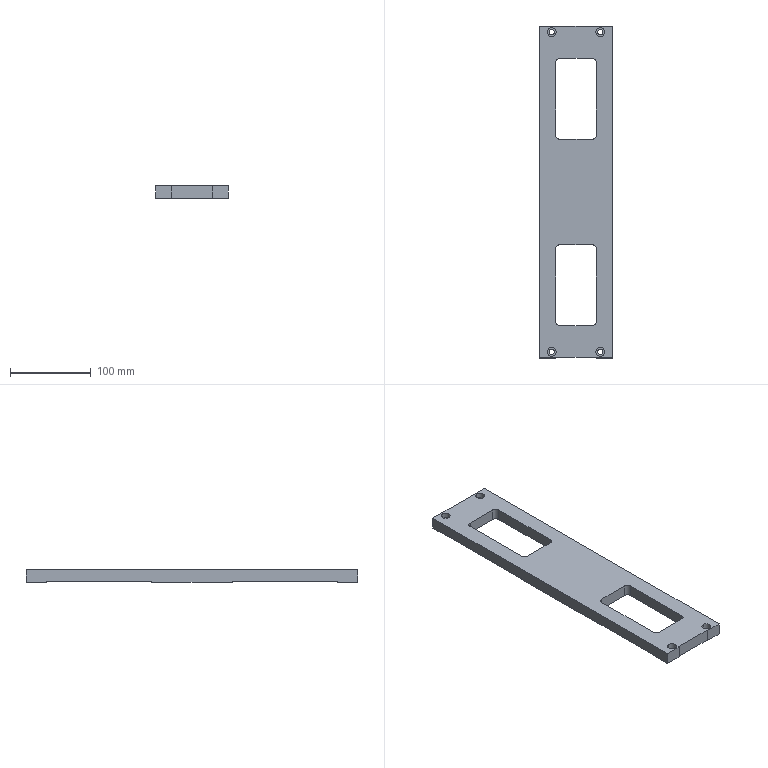NC program | NX | posted with a generic post | part box 90 x 410 x 15 mm
Lines 56 to 1434 of 4348:
(ZLEVEL_PROFILE , TOOL : D10)
N98 T10 M6
N100 G54
N102 G17 G0 G90 X209.1 Y-18.909 S9500 M3
N104 G43 Z30. H10
N106 Z1.5
N108 G94 G1 Y-21.967 Z1.34 F1000.
N110 X209.29 Y-22.224 Z1.323
N112 X209.699 Y-22.992 Z1.277
N114 X209.972 Y-23.819 Z1.232
N116 X210.1 Y-24.68 Z1.186
N118 Y-45.32 Z0.104
N120 X209.983 Y-46.131 Z0.062
N122 X209.738 Y-46.914 Z0.019
N124 X209.371 Y-47.647 Z-0.024
N126 X208.892 Y-48.312 Z-0.067
N128 X208.312 Y-48.892 Z-0.11
N130 X207.647 Y-49.371 Z-0.153
N132 X206.914 Y-49.738 Z-0.196
N134 X206.131 Y-49.983 Z-0.239
N136 X205.32 Y-50.1 Z-0.282
N138 X205. Z-0.299
N140 X-205. F3000.
N142 G2 X-210.1 Y-45. R5.1
N144 G1 Y45.
N146 G2 X-205. Y50.1 R5.1
N148 G1 X205.
N150 G2 X210.1 Y45. R5.1
N152 G1 Y25.
N154 G2 X209.1 Y21.967 R5.1
N156 G1 Y-21.967
N158 G2 X210.1 Y-25. R5.1
N160 G1 Y-45.
N162 G2 X205. Y-50.1 R5.1
N164 G1 X187.87 Z-0.598
N166 X-205.
N168 G2 X-210.1 Y-45. R5.1
N170 G1 Y45.
N172 G2 X-205. Y50.1 R5.1
N174 G1 X205.
N176 G2 X210.1 Y45. R5.1
N178 G1 Y25.
N180 G2 X209.1 Y21.967 R5.1
N182 G1 Y-21.967
N184 G2 X210.1 Y-25. R5.1
N186 G1 Y-45.
N188 G2 X205. Y-50.1 R5.1
N190 G1 X187.87 Z-0.897
N192 X-205.
N194 G2 X-210.1 Y-45. R5.1
N196 G1 Y45.
N198 G2 X-205. Y50.1 R5.1
N200 G1 X205.
N202 G2 X210.1 Y45. R5.1
N204 G1 Y25.
N206 G2 X209.1 Y21.967 R5.1
N208 G1 Y-21.967
N210 G2 X210.1 Y-25. R5.1
N212 G1 Y-45.
N214 G2 X205. Y-50.1 R5.1
N216 G1 X187.87 Z-1.196
N218 X-205.
N220 G2 X-210.1 Y-45. R5.1
N222 G1 Y45.
N224 G2 X-205. Y50.1 R5.1
N226 G1 X205.
N228 G2 X210.1 Y45. R5.1
N230 G1 Y25.
N232 G2 X209.1 Y21.967 R5.1
N234 G1 Y-21.967
N236 G2 X210.1 Y-25. R5.1
N238 G1 Y-45.
N240 G2 X205. Y-50.1 R5.1
N242 G1 X187.87 Z-1.495
N244 X-205.
N246 G2 X-210.1 Y-45. R5.1
N248 G1 Y45.
N250 G2 X-205. Y50.1 R5.1
N252 G1 X205.
N254 G2 X210.1 Y45. R5.1
N256 G1 Y25.
N258 G2 X209.1 Y21.967 R5.1
N260 G1 Y-21.967
N262 G2 X210.1 Y-25. R5.1
N264 G1 Y-45.
N266 G2 X205. Y-50.1 R5.1
N268 G1 X187.87 Z-1.794
N270 X-205.
N272 G2 X-210.1 Y-45. R5.1
N274 G1 Y45.
N276 G2 X-205. Y50.1 R5.1
N278 G1 X205.
N280 G2 X210.1 Y45. R5.1
N282 G1 Y25.
N284 G2 X209.1 Y21.967 R5.1
N286 G1 Y-21.967
N288 G2 X210.1 Y-25. R5.1
N290 G1 Y-45.
N292 G2 X205. Y-50.1 R5.1
N294 G1 X187.87 Z-2.093
N296 X-205.
N298 G2 X-210.1 Y-45. R5.1
N300 G1 Y45.
N302 G2 X-205. Y50.1 R5.1
N304 G1 X205.
N306 G2 X210.1 Y45. R5.1
N308 G1 Y25.
N310 G2 X209.1 Y21.967 R5.1
N312 G1 Y-21.967
N314 G2 X210.1 Y-25. R5.1
N316 G1 Y-45.
N318 G2 X205. Y-50.1 R5.1
N320 G1 X187.87 Z-2.392
N322 X-205.
N324 G2 X-210.1 Y-45. R5.1
N326 G1 Y45.
N328 G2 X-205. Y50.1 R5.1
N330 G1 X205.
N332 G2 X210.1 Y45. R5.1
N334 G1 Y25.
N336 G2 X209.1 Y21.967 R5.1
N338 G1 Y-21.967
N340 G2 X210.1 Y-25. R5.1
N342 G1 Y-45.
N344 G2 X205. Y-50.1 R5.1
N346 G1 X187.87 Z-2.691
N348 X-205.
N350 G2 X-210.1 Y-45. R5.1
N352 G1 Y45.
N354 G2 X-205. Y50.1 R5.1
N356 G1 X205.
N358 G2 X210.1 Y45. R5.1
N360 G1 Y25.
N362 G2 X209.1 Y21.967 R5.1
N364 G1 Y-21.967
N366 G2 X210.1 Y-25. R5.1
N368 G1 Y-45.
N370 G2 X205. Y-50.1 R5.1
N372 G1 X187.87 Z-2.99
N374 X-205.
N376 G2 X-210.1 Y-45. R5.1
N378 G1 Y45.
N380 G2 X-205. Y50.1 R5.1
N382 G1 X205.
N384 G2 X210.1 Y45. R5.1
N386 G1 Y25.
N388 G2 X209.1 Y21.967 R5.1
N390 G1 Y-21.967
N392 G2 X210.1 Y-25. R5.1
N394 G1 Y-45.
N396 G2 X205. Y-50.1 R5.1
N398 G1 X187.87 Z-3.289
N400 X-205.
N402 G2 X-210.1 Y-45. R5.1
N404 G1 Y45.
N406 G2 X-205. Y50.1 R5.1
N408 G1 X205.
N410 G2 X210.1 Y45. R5.1
N412 G1 Y25.
N414 G2 X209.1 Y21.967 R5.1
N416 G1 Y-21.967
N418 G2 X210.1 Y-25. R5.1
N420 G1 Y-45.
N422 G2 X205. Y-50.1 R5.1
N424 G1 X187.87 Z-3.588
N426 X-205.
N428 G2 X-210.1 Y-45. R5.1
N430 G1 Y45.
N432 G2 X-205. Y50.1 R5.1
N434 G1 X205.
N436 G2 X210.1 Y45. R5.1
N438 G1 Y25.
N440 G2 X209.1 Y21.967 R5.1
N442 G1 Y-21.967
N444 G2 X210.1 Y-25. R5.1
N446 G1 Y-45.
N448 G2 X205. Y-50.1 R5.1
N450 G1 X187.87 Z-3.887
N452 X-205.
N454 G2 X-210.1 Y-45. R5.1
N456 G1 Y45.
N458 G2 X-205. Y50.1 R5.1
N460 G1 X205.
N462 G2 X210.1 Y45. R5.1
N464 G1 Y25.
N466 G2 X209.1 Y21.967 R5.1
N468 G1 Y-21.967
N470 G2 X210.1 Y-25. R5.1
N472 G1 Y-45.
N474 G2 X205. Y-50.1 R5.1
N476 G1 X187.87 Z-4.186
N478 X-205.
N480 G2 X-210.1 Y-45. R5.1
N482 G1 Y45.
N484 G2 X-205. Y50.1 R5.1
N486 G1 X205.
N488 G2 X210.1 Y45. R5.1
N490 G1 Y25.
N492 G2 X209.1 Y21.967 R5.1
N494 G1 Y-21.967
N496 G2 X210.1 Y-25. R5.1
N498 G1 Y-45.
N500 G2 X205. Y-50.1 R5.1
N502 G1 X187.87 Z-4.485
N504 X-205.
N506 G2 X-210.1 Y-45. R5.1
N508 G1 Y45.
N510 G2 X-205. Y50.1 R5.1
N512 G1 X205.
N514 G2 X210.1 Y45. R5.1
N516 G1 Y25.
N518 G2 X209.1 Y21.967 R5.1
N520 G1 Y-21.967
N522 G2 X210.1 Y-25. R5.1
N524 G1 Y-45.
N526 G2 X205. Y-50.1 R5.1
N528 G1 X187.87 Z-4.784
N530 X-205.
N532 G2 X-210.1 Y-45. R5.1
N534 G1 Y45.
N536 G2 X-205. Y50.1 R5.1
N538 G1 X205.
N540 G2 X210.1 Y45. R5.1
N542 G1 Y25.
N544 G2 X209.1 Y21.967 R5.1
N546 G1 Y-21.967
N548 G2 X210.1 Y-25. R5.1
N550 G1 Y-45.
N552 G2 X205. Y-50.1 R5.1
N554 G1 X187.87 Z-5.083
N556 X-205.
N558 G2 X-210.1 Y-45. R5.1
N560 G1 Y45.
N562 G2 X-205. Y50.1 R5.1
N564 G1 X205.
N566 G2 X210.1 Y45. R5.1
N568 G1 Y25.
N570 G2 X209.1 Y21.967 R5.1
N572 G1 Y-21.967
N574 G2 X210.1 Y-25. R5.1
N576 G1 Y-45.
N578 G2 X205. Y-50.1 R5.1
N580 G1 X187.87 Z-5.382
N582 X-205.
N584 G2 X-210.1 Y-45. R5.1
N586 G1 Y45.
N588 G2 X-205. Y50.1 R5.1
N590 G1 X205.
N592 G2 X210.1 Y45. R5.1
N594 G1 Y25.
N596 G2 X209.1 Y21.967 R5.1
N598 G1 Y-21.967
N600 G2 X210.1 Y-25. R5.1
N602 G1 Y-45.
N604 G2 X205. Y-50.1 R5.1
N606 G1 X187.87 Z-5.681
N608 X-205.
N610 G2 X-210.1 Y-45. R5.1
N612 G1 Y45.
N614 G2 X-205. Y50.1 R5.1
N616 G1 X205.
N618 G2 X210.1 Y45. R5.1
N620 G1 Y25.
N622 G2 X209.1 Y21.967 R5.1
N624 G1 Y-21.967
N626 G2 X210.1 Y-25. R5.1
N628 G1 Y-45.
N630 G2 X205. Y-50.1 R5.1
N632 G1 X187.87 Z-5.98
N634 X-205.
N636 G2 X-210.1 Y-45. R5.1
N638 G1 Y45.
N640 G2 X-205. Y50.1 R5.1
N642 G1 X205.
N644 G2 X210.1 Y45. R5.1
N646 G1 Y25.
N648 G2 X209.1 Y21.967 R5.1
N650 G1 Y-21.967
N652 G2 X210.1 Y-25. R5.1
N654 G1 Y-45.
N656 G2 X205. Y-50.1 R5.1
N658 G1 X187.87 Z-6.279
N660 X-205.
N662 G2 X-210.1 Y-45. R5.1
N664 G1 Y45.
N666 G2 X-205. Y50.1 R5.1
N668 G1 X205.
N670 G2 X210.1 Y45. R5.1
N672 G1 Y25.
N674 G2 X209.1 Y21.967 R5.1
N676 G1 Y-21.967
N678 G2 X210.1 Y-25. R5.1
N680 G1 Y-45.
N682 G2 X205. Y-50.1 R5.1
N684 G1 X187.87 Z-6.578
N686 X-205.
N688 G2 X-210.1 Y-45. R5.1
N690 G1 Y45.
N692 G2 X-205. Y50.1 R5.1
N694 G1 X205.
N696 G2 X210.1 Y45. R5.1
N698 G1 Y25.
N700 G2 X209.1 Y21.967 R5.1
N702 G1 Y-21.967
N704 G2 X210.1 Y-25. R5.1
N706 G1 Y-45.
N708 G2 X205. Y-50.1 R5.1
N710 G1 X187.87 Z-6.877
N712 X-205.
N714 G2 X-210.1 Y-45. R5.1
N716 G1 Y45.
N718 G2 X-205. Y50.1 R5.1
N720 G1 X205.
N722 G2 X210.1 Y45. R5.1
N724 G1 Y25.
N726 G2 X209.1 Y21.967 R5.1
N728 G1 Y-21.967
N730 G2 X210.1 Y-25. R5.1
N732 G1 Y-45.
N734 G2 X205. Y-50.1 R5.1
N736 G1 X187.87 Z-7.176
N738 X-205.
N740 G2 X-210.1 Y-45. R5.1
N742 G1 Y45.
N744 G2 X-205. Y50.1 R5.1
N746 G1 X205.
N748 G2 X210.1 Y45. R5.1
N750 G1 Y25.
N752 G2 X209.1 Y21.967 R5.1
N754 G1 Y-21.967
N756 G2 X210.1 Y-25. R5.1
N758 G1 Y-45.
N760 G2 X205. Y-50.1 R5.1
N762 G1 X187.87 Z-7.475
N764 X-205.
N766 G2 X-210.1 Y-45. R5.1
N768 G1 Y45.
N770 G2 X-205. Y50.1 R5.1
N772 G1 X205.
N774 G2 X210.1 Y45. R5.1
N776 G1 Y25.
N778 G2 X209.1 Y21.967 R5.1
N780 G1 Y-21.967
N782 G2 X210.1 Y-25. R5.1
N784 G1 Y-45.
N786 G2 X205. Y-50.1 R5.1
N788 G1 X187.87 Z-7.774
N790 X-205.
N792 G2 X-210.1 Y-45. R5.1
N794 G1 Y45.
N796 G2 X-205. Y50.1 R5.1
N798 G1 X205.
N800 G2 X210.1 Y45. R5.1
N802 G1 Y25.
N804 G2 X209.1 Y21.967 R5.1
N806 G1 Y-21.967
N808 G2 X210.1 Y-25. R5.1
N810 G1 Y-45.
N812 G2 X205. Y-50.1 R5.1
N814 G1 X187.87 Z-8.073
N816 X-205.
N818 G2 X-210.1 Y-45. R5.1
N820 G1 Y45.
N822 G2 X-205. Y50.1 R5.1
N824 G1 X205.
N826 G2 X210.1 Y45. R5.1
N828 G1 Y25.
N830 G2 X209.1 Y21.967 R5.1
N832 G1 Y-21.967
N834 G2 X210.1 Y-25. R5.1
N836 G1 Y-45.
N838 G2 X205. Y-50.1 R5.1
N840 G1 X187.87 Z-8.372
N842 X-205.
N844 G2 X-210.1 Y-45. R5.1
N846 G1 Y45.
N848 G2 X-205. Y50.1 R5.1
N850 G1 X205.
N852 G2 X210.1 Y45. R5.1
N854 G1 Y25.
N856 G2 X209.1 Y21.967 R5.1
N858 G1 Y-21.967
N860 G2 X210.1 Y-25. R5.1
N862 G1 Y-45.
N864 G2 X205. Y-50.1 R5.1
N866 G1 X187.87 Z-8.671
N868 X-205.
N870 G2 X-210.1 Y-45. R5.1
N872 G1 Y45.
N874 G2 X-205. Y50.1 R5.1
N876 G1 X205.
N878 G2 X210.1 Y45. R5.1
N880 G1 Y25.
N882 G2 X209.1 Y21.967 R5.1
N884 G1 Y-21.967
N886 G2 X210.1 Y-25. R5.1
N888 G1 Y-45.
N890 G2 X205. Y-50.1 R5.1
N892 G1 X187.87 Z-8.97
N894 X-205.
N896 G2 X-210.1 Y-45. R5.1
N898 G1 Y45.
N900 G2 X-205. Y50.1 R5.1
N902 G1 X205.
N904 G2 X210.1 Y45. R5.1
N906 G1 Y25.
N908 G2 X209.1 Y21.967 R5.1
N910 G1 Y-21.967
N912 G2 X210.1 Y-25. R5.1
N914 G1 Y-45.
N916 G2 X205. Y-50.1 R5.1
N918 G1 X187.87 Z-9.269
N920 X-205.
N922 G2 X-210.1 Y-45. R5.1
N924 G1 Y45.
N926 G2 X-205. Y50.1 R5.1
N928 G1 X205.
N930 G2 X210.1 Y45. R5.1
N932 G1 Y25.
N934 G2 X209.1 Y21.967 R5.1
N936 G1 Y-21.967
N938 G2 X210.1 Y-25. R5.1
N940 G1 Y-45.
N942 G2 X205. Y-50.1 R5.1
N944 G1 X187.87 Z-9.568
N946 X-205.
N948 G2 X-210.1 Y-45. R5.1
N950 G1 Y45.
N952 G2 X-205. Y50.1 R5.1
N954 G1 X205.
N956 G2 X210.1 Y45. R5.1
N958 G1 Y25.
N960 G2 X209.1 Y21.967 R5.1
N962 G1 Y-21.967
N964 G2 X210.1 Y-25. R5.1
N966 G1 Y-45.
N968 G2 X205. Y-50.1 R5.1
N970 G1 X187.87 Z-9.867
N972 X-205.
N974 G2 X-210.1 Y-45. R5.1
N976 G1 Y45.
N978 G2 X-205. Y50.1 R5.1
N980 G1 X205.
N982 G2 X210.1 Y45. R5.1
N984 G1 Y25.
N986 G2 X209.1 Y21.967 R5.1
N988 G1 Y-21.967
N990 G2 X210.1 Y-25. R5.1
N992 G1 Y-45.
N994 G2 X205. Y-50.1 R5.1
N996 G1 X187.87 Z-10.166
N998 X-205.
N1000 G2 X-210.1 Y-45. R5.1
N1002 G1 Y45.
N1004 G2 X-205. Y50.1 R5.1
N1006 G1 X205.
N1008 G2 X210.1 Y45. R5.1
N1010 G1 Y25.
N1012 G2 X209.1 Y21.967 R5.1
N1014 G1 Y-21.967
N1016 G2 X210.1 Y-25. R5.1
N1018 G1 Y-45.
N1020 G2 X205. Y-50.1 R5.1
N1022 G1 X187.87 Z-10.465
N1024 X-205.
N1026 G2 X-210.1 Y-45. R5.1
N1028 G1 Y45.
N1030 G2 X-205. Y50.1 R5.1
N1032 G1 X205.
N1034 G2 X210.1 Y45. R5.1
N1036 G1 Y25.
N1038 G2 X209.1 Y21.967 R5.1
N1040 G1 Y-21.967
N1042 G2 X210.1 Y-25. R5.1
N1044 G1 Y-45.
N1046 G2 X205. Y-50.1 R5.1
N1048 G1 X187.87 Z-10.764
N1050 X-205.
N1052 G2 X-210.1 Y-45. R5.1
N1054 G1 Y45.
N1056 G2 X-205. Y50.1 R5.1
N1058 G1 X205.
N1060 G2 X210.1 Y45. R5.1
N1062 G1 Y25.
N1064 G2 X209.1 Y21.967 R5.1
N1066 G1 Y-21.967
N1068 G2 X210.1 Y-25. R5.1
N1070 G1 Y-45.
N1072 G2 X205. Y-50.1 R5.1
N1074 G1 X187.87 Z-11.063
N1076 X-205.
N1078 G2 X-210.1 Y-45. R5.1
N1080 G1 Y45.
N1082 G2 X-205. Y50.1 R5.1
N1084 G1 X205.
N1086 G2 X210.1 Y45. R5.1
N1088 G1 Y25.
N1090 G2 X209.1 Y21.967 R5.1
N1092 G1 Y-21.967
N1094 G2 X210.1 Y-25. R5.1
N1096 G1 Y-45.
N1098 G2 X205. Y-50.1 R5.1
N1100 G1 X187.87 Z-11.362
N1102 X-205.
N1104 G2 X-210.1 Y-45. R5.1
N1106 G1 Y45.
N1108 G2 X-205. Y50.1 R5.1
N1110 G1 X205.
N1112 G2 X210.1 Y45. R5.1
N1114 G1 Y25.
N1116 G2 X209.1 Y21.967 R5.1
N1118 G1 Y-21.967
N1120 G2 X210.1 Y-25. R5.1
N1122 G1 Y-45.
N1124 G2 X205. Y-50.1 R5.1
N1126 G1 X187.87 Z-11.661
N1128 X-205.
N1130 G2 X-210.1 Y-45. R5.1
N1132 G1 Y45.
N1134 G2 X-205. Y50.1 R5.1
N1136 G1 X205.
N1138 G2 X210.1 Y45. R5.1
N1140 G1 Y25.
N1142 G2 X209.1 Y21.967 R5.1
N1144 G1 Y-21.967
N1146 G2 X210.1 Y-25. R5.1
N1148 G1 Y-45.
N1150 G2 X205. Y-50.1 R5.1
N1152 G1 X187.87 Z-11.96
N1154 X-205.
N1156 G2 X-210.1 Y-45. R5.1
N1158 G1 Y45.
N1160 G2 X-205. Y50.1 R5.1
N1162 G1 X205.
N1164 G2 X210.1 Y45. R5.1
N1166 G1 Y25.
N1168 G2 X209.1 Y21.967 R5.1
N1170 G1 Y-21.967
N1172 G2 X210.1 Y-25. R5.1
N1174 G1 Y-45.
N1176 G2 X205. Y-50.1 R5.1
N1178 G1 X187.87 Z-12.259
N1180 X-205.
N1182 G2 X-210.1 Y-45. R5.1
N1184 G1 Y45.
N1186 G2 X-205. Y50.1 R5.1
N1188 G1 X205.
N1190 G2 X210.1 Y45. R5.1
N1192 G1 Y25.
N1194 G2 X209.1 Y21.967 R5.1
N1196 G1 Y-21.967
N1198 G2 X210.1 Y-25. R5.1
N1200 G1 Y-45.
N1202 G2 X205. Y-50.1 R5.1
N1204 G1 X187.87 Z-12.558
N1206 X-205.
N1208 G2 X-210.1 Y-45. R5.1
N1210 G1 Y45.
N1212 G2 X-205. Y50.1 R5.1
N1214 G1 X205.
N1216 G2 X210.1 Y45. R5.1
N1218 G1 Y25.
N1220 G2 X209.1 Y21.967 R5.1
N1222 G1 Y-21.967
N1224 G2 X210.1 Y-25. R5.1
N1226 G1 Y-45.
N1228 G2 X205. Y-50.1 R5.1
N1230 G1 X187.87 Z-12.857
N1232 X-205.
N1234 G2 X-210.1 Y-45. R5.1
N1236 G1 Y45.
N1238 G2 X-205. Y50.1 R5.1
N1240 G1 X205.
N1242 G2 X210.1 Y45. R5.1
N1244 G1 Y25.
N1246 G2 X209.1 Y21.967 R5.1
N1248 G1 Y-21.967
N1250 G2 X210.1 Y-25. R5.1
N1252 G1 Y-45.
N1254 G2 X205. Y-50.1 R5.1
N1256 G1 X187.87 Z-13.156
N1258 X-205.
N1260 G2 X-210.1 Y-45. R5.1
N1262 G1 Y45.
N1264 G2 X-205. Y50.1 R5.1
N1266 G1 X205.
N1268 G2 X210.1 Y45. R5.1
N1270 G1 Y25.
N1272 G2 X209.1 Y21.967 R5.1
N1274 G1 Y-21.967
N1276 G2 X210.1 Y-25. R5.1
N1278 G1 Y-45.
N1280 G2 X205. Y-50.1 R5.1
N1282 G1 X187.87 Z-13.455
N1284 X-205.
N1286 G2 X-210.1 Y-45. R5.1
N1288 G1 Y45.
N1290 G2 X-205. Y50.1 R5.1
N1292 G1 X205.
N1294 G2 X210.1 Y45. R5.1
N1296 G1 Y25.
N1298 G2 X209.1 Y21.967 R5.1
N1300 G1 Y-21.967
N1302 G2 X210.1 Y-25. R5.1
N1304 G1 Y-45.
N1306 G2 X205. Y-50.1 R5.1
N1308 G1 X187.87 Z-13.754
N1310 X-205.
N1312 G2 X-210.1 Y-45. R5.1
N1314 G1 Y45.
N1316 G2 X-205. Y50.1 R5.1
N1318 G1 X205.
N1320 G2 X210.1 Y45. R5.1
N1322 G1 Y25.
N1324 G2 X209.1 Y21.967 R5.1
N1326 G1 Y-21.967
N1328 G2 X210.1 Y-25. R5.1
N1330 G1 Y-45.
N1332 G2 X205. Y-50.1 R5.1
N1334 G1 X187.87 Z-14.053
N1336 X-205.
N1338 G2 X-210.1 Y-45. R5.1
N1340 G1 Y45.
N1342 G2 X-205. Y50.1 R5.1
N1344 G1 X205.
N1346 G2 X210.1 Y45. R5.1
N1348 G1 Y25.
N1350 G2 X209.1 Y21.967 R5.1
N1352 G1 Y-21.967
N1354 G2 X210.1 Y-25. R5.1
N1356 G1 Y-45.
N1358 G2 X205. Y-50.1 R5.1
N1360 G1 X187.87 Z-14.352
N1362 X-205.
N1364 G2 X-210.1 Y-45. R5.1
N1366 G1 Y45.
N1368 G2 X-205. Y50.1 R5.1
N1370 G1 X205.
N1372 G2 X210.1 Y45. R5.1
N1374 G1 Y25.
N1376 G2 X209.1 Y21.967 R5.1
N1378 G1 Y-21.967
N1380 G2 X210.1 Y-25. R5.1
N1382 G1 Y-45.
N1384 G2 X205. Y-50.1 R5.1
N1386 G1 X187.87 Z-14.651
N1388 X-205.
N1390 G2 X-210.1 Y-45. R5.1
N1392 G1 Y45.
N1394 G2 X-205. Y50.1 R5.1
N1396 G1 X205.
N1398 G2 X210.1 Y45. R5.1
N1400 G1 Y25.
N1402 G2 X209.1 Y21.967 R5.1
N1404 G1 Y-21.967
N1406 G2 X210.1 Y-25. R5.1
N1408 G1 Y-45.
N1410 G2 X205. Y-50.1 R5.1
N1412 G1 X187.87 Z-14.95
N1414 X-205.
N1416 G2 X-210.1 Y-45. R5.1
N1418 G1 Y45.
N1420 G2 X-205. Y50.1 R5.1
N1422 G1 X205.
N1424 G2 X210.1 Y45. R5.1
N1426 G1 Y25.
N1428 G2 X209.1 Y21.967 R5.1
N1430 G1 Y-21.967
N1432 G2 X210.1 Y-25. R5.1
N1434 G1 Y-45.
N1436 G2 X205. Y-50.1 R5.1
N1438 G1 X187.87
N1440 Z-13.45
N1442 G0 Z30.
(PLANAR_MILL , TOOL : D10)
N1444 X-134.081 Y-1.9
N1446 Z0.7
N1448 G1 X-115. Z-0.3 F1000.
N1450 X-88.1 F3000.
N1452 Y1.9
N1454 X-141.9
N1456 Y-1.9
N1458 X-115.
N1460 Y-7.9
N1462 X-82.1
N1464 Y7.9
N1466 X-147.9
N1468 Y-7.9
N1470 X-115.
N1472 Y-13.9
N1474 X-76.1
N1476 Y13.9
N1478 X-153.9
N1480 Y-13.9
N1482 X-115.
N1484 Y-19.9
N1486 X-70.1
N1488 Y19.9
N1490 X-159.9
N1492 Y-19.9
N1494 X-115.
N1496 Z0.4
N1498 G0 X-134.081 Y-1.9
N1500 G1 X-115. Z-0.6 F1000.
N1502 X-88.1 F3000.
N1504 Y1.9
N1506 X-141.9
N1508 Y-1.9
N1510 X-115.
N1512 Y-7.9
N1514 X-82.1
N1516 Y7.9
N1518 X-147.9
N1520 Y-7.9
N1522 X-115.
N1524 Y-13.9
N1526 X-76.1
N1528 Y13.9
N1530 X-153.9
N1532 Y-13.9
N1534 X-115.
N1536 Y-19.9
N1538 X-70.1
N1540 Y19.9
N1542 X-159.9
N1544 Y-19.9
N1546 X-115.
N1548 Z0.1
N1550 G0 X-134.081 Y-1.9
N1552 G1 X-115. Z-0.9 F1000.
N1554 X-88.1 F3000.
N1556 Y1.9
N1558 X-141.9
N1560 Y-1.9
N1562 X-115.
N1564 Y-7.9
N1566 X-82.1
N1568 Y7.9
N1570 X-147.9
N1572 Y-7.9
N1574 X-115.
N1576 Y-13.9
N1578 X-76.1
N1580 Y13.9
N1582 X-153.9
N1584 Y-13.9
N1586 X-115.
N1588 Y-19.9
N1590 X-70.1
N1592 Y19.9
N1594 X-159.9
N1596 Y-19.9
N1598 X-115.
N1600 Z-0.2
N1602 G0 X-134.081 Y-1.9
N1604 G1 X-115. Z-1.2 F1000.
N1606 X-88.1 F3000.
N1608 Y1.9
N1610 X-141.9
N1612 Y-1.9
N1614 X-115.
N1616 Y-7.9
N1618 X-82.1
N1620 Y7.9
N1622 X-147.9
N1624 Y-7.9
N1626 X-115.
N1628 Y-13.9
N1630 X-76.1
N1632 Y13.9
N1634 X-153.9
N1636 Y-13.9
N1638 X-115.
N1640 Y-19.9
N1642 X-70.1
N1644 Y19.9
N1646 X-159.9
N1648 Y-19.9
N1650 X-115.
N1652 Z-0.5
N1654 G0 X-134.081 Y-1.9
N1656 G1 X-115. Z-1.5 F1000.
N1658 X-88.1 F3000.
N1660 Y1.9
N1662 X-141.9
N1664 Y-1.9
N1666 X-115.
N1668 Y-7.9
N1670 X-82.1
N1672 Y7.9
N1674 X-147.9
N1676 Y-7.9
N1678 X-115.
N1680 Y-13.9
N1682 X-76.1
N1684 Y13.9
N1686 X-153.9
N1688 Y-13.9
N1690 X-115.
N1692 Y-19.9
N1694 X-70.1
N1696 Y19.9
N1698 X-159.9
N1700 Y-19.9
N1702 X-115.
N1704 Z-0.8
N1706 G0 X-134.081 Y-1.9
N1708 G1 X-115. Z-1.8 F1000.
N1710 X-88.1 F3000.
N1712 Y1.9
N1714 X-141.9
N1716 Y-1.9
N1718 X-115.
N1720 Y-7.9
N1722 X-82.1
N1724 Y7.9
N1726 X-147.9
N1728 Y-7.9
N1730 X-115.
N1732 Y-13.9
N1734 X-76.1
N1736 Y13.9
N1738 X-153.9
N1740 Y-13.9
N1742 X-115.
N1744 Y-19.9
N1746 X-70.1
N1748 Y19.9
N1750 X-159.9
N1752 Y-19.9
N1754 X-115.
N1756 Z-1.1
N1758 G0 X-134.081 Y-1.9
N1760 G1 X-115. Z-2.1 F1000.
N1762 X-88.1 F3000.
N1764 Y1.9
N1766 X-141.9
N1768 Y-1.9
N1770 X-115.
N1772 Y-7.9
N1774 X-82.1
N1776 Y7.9
N1778 X-147.9
N1780 Y-7.9
N1782 X-115.
N1784 Y-13.9
N1786 X-76.1
N1788 Y13.9
N1790 X-153.9
N1792 Y-13.9
N1794 X-115.
N1796 Y-19.9
N1798 X-70.1
N1800 Y19.9
N1802 X-159.9
N1804 Y-19.9
N1806 X-115.
N1808 Z-1.4
N1810 G0 X-134.081 Y-1.9
N1812 G1 X-115. Z-2.4 F1000.
N1814 X-88.1 F3000.
N1816 Y1.9
N1818 X-141.9
N1820 Y-1.9
N1822 X-115.
N1824 Y-7.9
N1826 X-82.1
N1828 Y7.9
N1830 X-147.9
N1832 Y-7.9
N1834 X-115.
N1836 Y-13.9
N1838 X-76.1
N1840 Y13.9
N1842 X-153.9
N1844 Y-13.9
N1846 X-115.
N1848 Y-19.9
N1850 X-70.1
N1852 Y19.9
N1854 X-159.9
N1856 Y-19.9
N1858 X-115.
N1860 Z-1.7
N1862 G0 X-134.081 Y-1.9
N1864 G1 X-115. Z-2.7 F1000.
N1866 X-88.1 F3000.
N1868 Y1.9
N1870 X-141.9
N1872 Y-1.9
N1874 X-115.
N1876 Y-7.9
N1878 X-82.1
N1880 Y7.9
N1882 X-147.9
N1884 Y-7.9
N1886 X-115.
N1888 Y-13.9
N1890 X-76.1
N1892 Y13.9
N1894 X-153.9
N1896 Y-13.9
N1898 X-115.
N1900 Y-19.9
N1902 X-70.1
N1904 Y19.9
N1906 X-159.9
N1908 Y-19.9
N1910 X-115.
N1912 Z-2.
N1914 G0 X-134.081 Y-1.9
N1916 G1 X-115. Z-3. F1000.
N1918 X-88.1 F3000.
N1920 Y1.9
N1922 X-141.9
N1924 Y-1.9
N1926 X-115.
N1928 Y-7.9
N1930 X-82.1
N1932 Y7.9
N1934 X-147.9
N1936 Y-7.9
N1938 X-115.
N1940 Y-13.9
N1942 X-76.1
N1944 Y13.9
N1946 X-153.9
N1948 Y-13.9
N1950 X-115.
N1952 Y-19.9
N1954 X-70.1
N1956 Y19.9
N1958 X-159.9
N1960 Y-19.9
N1962 X-115.
N1964 Z-2.3
N1966 G0 X-134.081 Y-1.9
N1968 G1 X-115. Z-3.3 F1000.
N1970 X-88.1 F3000.
N1972 Y1.9
N1974 X-141.9
N1976 Y-1.9
N1978 X-115.
N1980 Y-7.9
N1982 X-82.1
N1984 Y7.9
N1986 X-147.9
N1988 Y-7.9
N1990 X-115.
N1992 Y-13.9
N1994 X-76.1
N1996 Y13.9
N1998 X-153.9
N2000 Y-13.9
N2002 X-115.
N2004 Y-19.9
N2006 X-70.1
N2008 Y19.9
N2010 X-159.9
N2012 Y-19.9
N2014 X-115.
N2016 Z-2.6
N2018 G0 X-134.081 Y-1.9
N2020 G1 X-115. Z-3.6 F1000.
N2022 X-88.1 F3000.
N2024 Y1.9
N2026 X-141.9
N2028 Y-1.9
N2030 X-115.
N2032 Y-7.9
N2034 X-82.1
N2036 Y7.9
N2038 X-147.9
N2040 Y-7.9
N2042 X-115.
N2044 Y-13.9
N2046 X-76.1
N2048 Y13.9
N2050 X-153.9
N2052 Y-13.9
N2054 X-115.
N2056 Y-19.9
N2058 X-70.1
N2060 Y19.9
N2062 X-159.9
N2064 Y-19.9
N2066 X-115.
N2068 Z-2.9
N2070 G0 X-134.081 Y-1.9
N2072 G1 X-115. Z-3.9 F1000.
N2074 X-88.1 F3000.
N2076 Y1.9
N2078 X-141.9
N2080 Y-1.9
N2082 X-115.
N2084 Y-7.9
N2086 X-82.1
N2088 Y7.9
N2090 X-147.9
N2092 Y-7.9
N2094 X-115.
N2096 Y-13.9
N2098 X-76.1
N2100 Y13.9
N2102 X-153.9
N2104 Y-13.9
N2106 X-115.
N2108 Y-19.9
N2110 X-70.1
N2112 Y19.9
N2114 X-159.9
N2116 Y-19.9
N2118 X-115.
N2120 Z-3.2
N2122 G0 X-134.081 Y-1.9
N2124 G1 X-115. Z-4.2 F1000.
N2126 X-88.1 F3000.
N2128 Y1.9
N2130 X-141.9
N2132 Y-1.9
N2134 X-115.
N2136 Y-7.9
N2138 X-82.1
N2140 Y7.9
N2142 X-147.9
N2144 Y-7.9
N2146 X-115.
N2148 Y-13.9
N2150 X-76.1
N2152 Y13.9
N2154 X-153.9
N2156 Y-13.9
N2158 X-115.
N2160 Y-19.9
N2162 X-70.1
N2164 Y19.9
N2166 X-159.9
N2168 Y-19.9
N2170 X-115.
N2172 Z-3.5
N2174 G0 X-134.081 Y-1.9
N2176 G1 X-115. Z-4.5 F1000.
N2178 X-88.1 F3000.
N2180 Y1.9
N2182 X-141.9
N2184 Y-1.9
N2186 X-115.
N2188 Y-7.9
N2190 X-82.1
N2192 Y7.9
N2194 X-147.9
N2196 Y-7.9
N2198 X-115.
N2200 Y-13.9
N2202 X-76.1
N2204 Y13.9
N2206 X-153.9
N2208 Y-13.9
N2210 X-115.
N2212 Y-19.9
N2214 X-70.1
N2216 Y19.9
N2218 X-159.9
N2220 Y-19.9
N2222 X-115.
N2224 Z-3.8
N2226 G0 X-134.081 Y-1.9
N2228 G1 X-115. Z-4.8 F1000.
N2230 X-88.1 F3000.
N2232 Y1.9
N2234 X-141.9
N2236 Y-1.9
N2238 X-115.
N2240 Y-7.9
N2242 X-82.1
N2244 Y7.9
N2246 X-147.9
N2248 Y-7.9
N2250 X-115.
N2252 Y-13.9
N2254 X-76.1
N2256 Y13.9
N2258 X-153.9
N2260 Y-13.9
N2262 X-115.
N2264 Y-19.9
N2266 X-70.1
N2268 Y19.9
N2270 X-159.9
N2272 Y-19.9
N2274 X-115.
N2276 Z-4.1
N2278 G0 X-134.081 Y-1.9
N2280 G1 X-115. Z-5.1 F1000.
N2282 X-88.1 F3000.
N2284 Y1.9
N2286 X-141.9
N2288 Y-1.9
N2290 X-115.
N2292 Y-7.9
N2294 X-82.1
N2296 Y7.9
N2298 X-147.9
N2300 Y-7.9
N2302 X-115.
N2304 Y-13.9
N2306 X-76.1
N2308 Y13.9
N2310 X-153.9
N2312 Y-13.9
N2314 X-115.
N2316 Y-19.9
N2318 X-70.1
N2320 Y19.9
N2322 X-159.9
N2324 Y-19.9
N2326 X-115.
N2328 Z-4.4
N2330 G0 X-134.081 Y-1.9
N2332 G1 X-115. Z-5.4 F1000.
N2334 X-88.1 F3000.
N2336 Y1.9
N2338 X-141.9
N2340 Y-1.9
N2342 X-115.
N2344 Y-7.9
N2346 X-82.1
N2348 Y7.9
N2350 X-147.9
N2352 Y-7.9
N2354 X-115.
N2356 Y-13.9
N2358 X-76.1
N2360 Y13.9
N2362 X-153.9
N2364 Y-13.9
N2366 X-115.
N2368 Y-19.9
N2370 X-70.1
N2372 Y19.9
N2374 X-159.9
N2376 Y-19.9
N2378 X-115.
N2380 Z-4.7
N2382 G0 X-134.081 Y-1.9
N2384 G1 X-115. Z-5.7 F1000.
N2386 X-88.1 F3000.
N2388 Y1.9
N2390 X-141.9
N2392 Y-1.9
N2394 X-115.
N2396 Y-7.9
N2398 X-82.1
N2400 Y7.9
N2402 X-147.9
N2404 Y-7.9
N2406 X-115.
N2408 Y-13.9
N2410 X-76.1
N2412 Y13.9
N2414 X-153.9
N2416 Y-13.9
N2418 X-115.
N2420 Y-19.9
N2422 X-70.1
N2424 Y19.9
N2426 X-159.9
N2428 Y-19.9
N2430 X-115.
N2432 Z-5.
N2434 G0 X-134.081 Y-1.9
N2436 G1 X-115. Z-6. F1000.
N2438 X-88.1 F3000.
N2440 Y1.9
N2442 X-141.9
N2444 Y-1.9
N2446 X-115.
N2448 Y-7.9
N2450 X-82.1
N2452 Y7.9
N2454 X-147.9
N2456 Y-7.9
N2458 X-115.
N2460 Y-13.9
N2462 X-76.1
N2464 Y13.9
N2466 X-153.9
N2468 Y-13.9
N2470 X-115.
N2472 Y-19.9
N2474 X-70.1
N2476 Y19.9
N2478 X-159.9
N2480 Y-19.9
N2482 X-115.
N2484 Z-5.3
N2486 G0 X-134.081 Y-1.9
N2488 G1 X-115. Z-6.3 F1000.
N2490 X-88.1 F3000.
N2492 Y1.9
N2494 X-141.9
N2496 Y-1.9
N2498 X-115.
N2500 Y-7.9
N2502 X-82.1
N2504 Y7.9
N2506 X-147.9
N2508 Y-7.9
N2510 X-115.
N2512 Y-13.9
N2514 X-76.1
N2516 Y13.9
N2518 X-153.9
N2520 Y-13.9
N2522 X-115.
N2524 Y-19.9
N2526 X-70.1
N2528 Y19.9
N2530 X-159.9
N2532 Y-19.9
N2534 X-115.
N2536 Z-5.6
N2538 G0 X-134.081 Y-1.9
N2540 G1 X-115. Z-6.6 F1000.
N2542 X-88.1 F3000.
N2544 Y1.9
N2546 X-141.9
N2548 Y-1.9
N2550 X-115.
N2552 Y-7.9
N2554 X-82.1
N2556 Y7.9
N2558 X-147.9
N2560 Y-7.9
N2562 X-115.
N2564 Y-13.9
N2566 X-76.1
N2568 Y13.9
N2570 X-153.9
N2572 Y-13.9
N2574 X-115.
N2576 Y-19.9
N2578 X-70.1
N2580 Y19.9
N2582 X-159.9
N2584 Y-19.9
N2586 X-115.
N2588 Z-5.9
N2590 G0 X-134.081 Y-1.9
N2592 G1 X-115. Z-6.9 F1000.
N2594 X-88.1 F3000.
N2596 Y1.9
N2598 X-141.9
N2600 Y-1.9
N2602 X-115.
N2604 Y-7.9
N2606 X-82.1
N2608 Y7.9
N2610 X-147.9
N2612 Y-7.9
N2614 X-115.
N2616 Y-13.9
N2618 X-76.1
N2620 Y13.9
N2622 X-153.9
N2624 Y-13.9
N2626 X-115.
N2628 Y-19.9
N2630 X-70.1
N2632 Y19.9
N2634 X-159.9
N2636 Y-19.9
N2638 X-115.
N2640 Z-6.2
N2642 G0 X-134.081 Y-1.9
N2644 G1 X-115. Z-7.2 F1000.
N2646 X-88.1 F3000.
N2648 Y1.9
N2650 X-141.9
N2652 Y-1.9
N2654 X-115.
N2656 Y-7.9
N2658 X-82.1
N2660 Y7.9
N2662 X-147.9
N2664 Y-7.9
N2666 X-115.
N2668 Y-13.9
N2670 X-76.1
N2672 Y13.9
N2674 X-153.9
N2676 Y-13.9
N2678 X-115.
N2680 Y-19.9
N2682 X-70.1
N2684 Y19.9
N2686 X-159.9
N2688 Y-19.9
N2690 X-115.
N2692 Z-6.5
N2694 G0 X-134.081 Y-1.9
N2696 G1 X-115. Z-7.5 F1000.
N2698 X-88.1 F3000.
N2700 Y1.9
N2702 X-141.9
N2704 Y-1.9
N2706 X-115.
N2708 Y-7.9
N2710 X-82.1
N2712 Y7.9
N2714 X-147.9
N2716 Y-7.9
N2718 X-115.
N2720 Y-13.9
N2722 X-76.1
N2724 Y13.9
N2726 X-153.9
N2728 Y-13.9
N2730 X-115.
N2732 Y-19.9
N2734 X-70.1
N2736 Y19.9
N2738 X-159.9
N2740 Y-19.9
N2742 X-115.
N2744 Z-6.8
N2746 G0 X-134.081 Y-1.9
N2748 G1 X-115. Z-7.8 F1000.
N2750 X-88.1 F3000.
N2752 Y1.9
N2754 X-141.9
N2756 Y-1.9
N2758 X-115.
N2760 Y-7.9
N2762 X-82.1
N2764 Y7.9
N2766 X-147.9
N2768 Y-7.9
N2770 X-115.
N2772 Y-13.9
N2774 X-76.1
N2776 Y13.9
N2778 X-153.9
N2780 Y-13.9
N2782 X-115.
N2784 Y-19.9
N2786 X-70.1
N2788 Y19.9
N2790 X-159.9
N2792 Y-19.9
N2794 X-115.
N2796 Z-7.1
N2798 G0 X-134.081 Y-1.9
N2800 G1 X-115. Z-8.1 F1000.
N2802 X-88.1 F3000.
N2804 Y1.9
N2806 X-141.9
N2808 Y-1.9
N2810 X-115.
N2812 Y-7.9
N2814 X-82.1
N2816 Y7.9
N2818 X-147.9
N2820 Y-7.9
N2822 X-115.
N2824 Y-13.9
N2826 X-76.1
N2828 Y13.9
N2830 X-153.9
N2832 Y-13.9
N2834 X-115.
N2836 Y-19.9
N2838 X-70.1
N2840 Y19.9
N2842 X-159.9